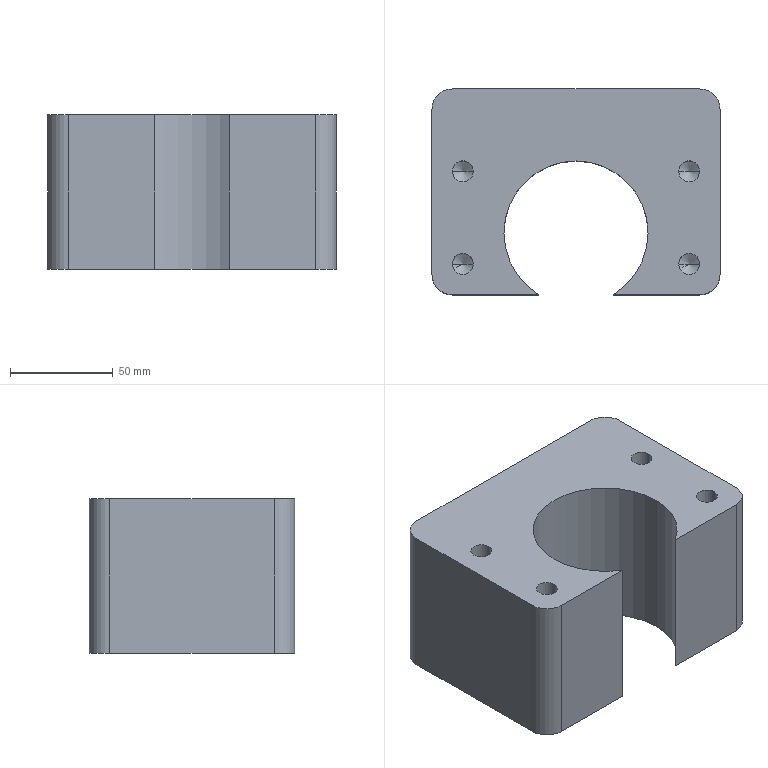Part | SolidWorks | features BaseBody 1 | 1 solid | 46 faces | box 140 x 100 x 75 mm | volume 742034 mm3 | cylinder 23 | cone 16 | plane 7 | commonest cylinder face diameters 8.5 x8 10.2 x8 20 x4 70 x3
STEP:
#1=CARTESIAN_POINT('',(-50.,40.,10.75));
#2=VERTEX_POINT('',#1);
#3=CARTESIAN_POINT('',(-50.,40.,19.25));
#4=VERTEX_POINT('',#3);
#5=CARTESIAN_POINT('',(-50.,40.,15.));
#6=DIRECTION('',(0.,1.,0.));
#7=DIRECTION('',(0.,0.,1.));
#8=AXIS2_PLACEMENT_3D('',#5,#6,#7);
#9=CIRCLE('',#8,4.25);
#10=EDGE_CURVE('',#2,#4,#9,.T.);
#11=ORIENTED_EDGE('',*,*,#10,.F.);
#12=CARTESIAN_POINT('',(-50.,70.,10.75));
#13=VERTEX_POINT('',#12);
#14=CARTESIAN_POINT('',(-50.,70.,10.75));
#15=DIRECTION('',(0.,1.,0.));
#16=VECTOR('',#15,1000.);
#17=LINE('',#14,#16);
#18=EDGE_CURVE('',#2,#13,#17,.T.);
#19=ORIENTED_EDGE('',*,*,#18,.T.);
#20=CARTESIAN_POINT('',(-50.,70.,19.25));
#21=VERTEX_POINT('',#20);
#22=CARTESIAN_POINT('',(-50.,70.,15.));
#23=DIRECTION('',(0.,1.,0.));
#24=DIRECTION('',(0.,0.,1.));
#25=AXIS2_PLACEMENT_3D('',#22,#23,#24);
#26=CIRCLE('',#25,4.25);
#27=EDGE_CURVE('',#13,#21,#26,.T.);
#28=ORIENTED_EDGE('',*,*,#27,.T.);
#29=CARTESIAN_POINT('',(-50.,70.,19.25));
#30=DIRECTION('',(0.,1.,0.));
#31=VECTOR('',#30,1000.);
#32=LINE('',#29,#31);
#33=EDGE_CURVE('',#4,#21,#32,.T.);
#34=ORIENTED_EDGE('',*,*,#33,.F.);
#35=EDGE_LOOP('',(#11,#19,#28,#34));
#36=FACE_OUTER_BOUND('',#35,.T.);
#37=CARTESIAN_POINT('',(-50.,70.,15.));
#38=DIRECTION('',(0.,1.,0.));
#39=DIRECTION('',(0.,0.,1.));
#40=AXIS2_PLACEMENT_3D('',#37,#38,#39);
#41=CYLINDRICAL_SURFACE('',#40,4.25);
#42=ADVANCED_FACE('',(#36),#41,.F.);
#43=CARTESIAN_POINT('',(-50.,37.446,15.));
#44=VERTEX_POINT('',#43);
#45=CARTESIAN_POINT('',(-50.,40.,19.25));
#46=DIRECTION('',(0.,0.515,0.8572));
#47=VECTOR('',#46,1000.);
#48=LINE('',#45,#47);
#49=EDGE_CURVE('',#44,#4,#48,.T.);
#50=ORIENTED_EDGE('',*,*,#49,.F.);
#51=CARTESIAN_POINT('',(-50.,40.,10.75));
#52=DIRECTION('',(0.,0.515,-0.8572));
#53=VECTOR('',#52,1000.);
#54=LINE('',#51,#53);
#55=EDGE_CURVE('',#44,#2,#54,.T.);
#56=ORIENTED_EDGE('',*,*,#55,.T.);
#57=ORIENTED_EDGE('',*,*,#10,.T.);
#58=EDGE_LOOP('',(#50,#56,#57));
#59=FACE_OUTER_BOUND('',#58,.T.);
#60=CARTESIAN_POINT('',(-50.,40.,15.));
#61=DIRECTION('',(0.,1.,0.));
#62=DIRECTION('',(0.,0.,1.));
#63=AXIS2_PLACEMENT_3D('',#60,#61,#62);
#64=CONICAL_SURFACE('',#63,4.25,1.03);
#65=ADVANCED_FACE('',(#59),#64,.F.);
#66=CARTESIAN_POINT('',(-50.,40.,50.75));
#67=VERTEX_POINT('',#66);
#68=CARTESIAN_POINT('',(-50.,40.,59.25));
#69=VERTEX_POINT('',#68);
#70=CARTESIAN_POINT('',(-50.,40.,55.));
#71=DIRECTION('',(0.,1.,0.));
#72=DIRECTION('',(0.,0.,1.));
#73=AXIS2_PLACEMENT_3D('',#70,#71,#72);
#74=CIRCLE('',#73,4.25);
#75=EDGE_CURVE('',#67,#69,#74,.T.);
#76=ORIENTED_EDGE('',*,*,#75,.F.);
#77=CARTESIAN_POINT('',(-50.,70.,50.75));
#78=VERTEX_POINT('',#77);
#79=CARTESIAN_POINT('',(-50.,70.,50.75));
#80=DIRECTION('',(0.,1.,0.));
#81=VECTOR('',#80,1000.);
#82=LINE('',#79,#81);
#83=EDGE_CURVE('',#67,#78,#82,.T.);
#84=ORIENTED_EDGE('',*,*,#83,.T.);
#85=CARTESIAN_POINT('',(-50.,70.,59.25));
#86=VERTEX_POINT('',#85);
#87=CARTESIAN_POINT('',(-50.,70.,55.));
#88=DIRECTION('',(0.,1.,0.));
#89=DIRECTION('',(0.,0.,1.));
#90=AXIS2_PLACEMENT_3D('',#87,#88,#89);
#91=CIRCLE('',#90,4.25);
#92=EDGE_CURVE('',#78,#86,#91,.T.);
#93=ORIENTED_EDGE('',*,*,#92,.T.);
#94=CARTESIAN_POINT('',(-50.,70.,59.25));
#95=DIRECTION('',(0.,1.,0.));
#96=VECTOR('',#95,1000.);
#97=LINE('',#94,#96);
#98=EDGE_CURVE('',#69,#86,#97,.T.);
#99=ORIENTED_EDGE('',*,*,#98,.F.);
#100=EDGE_LOOP('',(#76,#84,#93,#99));
#101=FACE_OUTER_BOUND('',#100,.T.);
#102=CARTESIAN_POINT('',(-50.,70.,55.));
#103=DIRECTION('',(0.,1.,0.));
#104=DIRECTION('',(0.,0.,1.));
#105=AXIS2_PLACEMENT_3D('',#102,#103,#104);
#106=CYLINDRICAL_SURFACE('',#105,4.25);
#107=ADVANCED_FACE('',(#101),#106,.F.);
#108=CARTESIAN_POINT('',(-50.,37.446,55.));
#109=VERTEX_POINT('',#108);
#110=CARTESIAN_POINT('',(-50.,40.,59.25));
#111=DIRECTION('',(0.,0.515,0.8572));
#112=VECTOR('',#111,1000.);
#113=LINE('',#110,#112);
#114=EDGE_CURVE('',#109,#69,#113,.T.);
#115=ORIENTED_EDGE('',*,*,#114,.F.);
#116=CARTESIAN_POINT('',(-50.,40.,50.75));
#117=DIRECTION('',(0.,0.515,-0.8572));
#118=VECTOR('',#117,1000.);
#119=LINE('',#116,#118);
#120=EDGE_CURVE('',#109,#67,#119,.T.);
#121=ORIENTED_EDGE('',*,*,#120,.T.);
#122=ORIENTED_EDGE('',*,*,#75,.T.);
#123=EDGE_LOOP('',(#115,#121,#122));
#124=FACE_OUTER_BOUND('',#123,.T.);
#125=CARTESIAN_POINT('',(-50.,40.,55.));
#126=DIRECTION('',(0.,1.,0.));
#127=DIRECTION('',(0.,0.,1.));
#128=AXIS2_PLACEMENT_3D('',#125,#126,#127);
#129=CONICAL_SURFACE('',#128,4.25,1.03);
#130=ADVANCED_FACE('',(#124),#129,.F.);
#131=CARTESIAN_POINT('',(50.,40.,50.75));
#132=VERTEX_POINT('',#131);
#133=CARTESIAN_POINT('',(50.,40.,59.25));
#134=VERTEX_POINT('',#133);
#135=CARTESIAN_POINT('',(50.,40.,55.));
#136=DIRECTION('',(0.,1.,0.));
#137=DIRECTION('',(0.,0.,1.));
#138=AXIS2_PLACEMENT_3D('',#135,#136,#137);
#139=CIRCLE('',#138,4.25);
#140=EDGE_CURVE('',#132,#134,#139,.T.);
#141=ORIENTED_EDGE('',*,*,#140,.F.);
#142=CARTESIAN_POINT('',(50.,70.,50.75));
#143=VERTEX_POINT('',#142);
#144=CARTESIAN_POINT('',(50.,70.,50.75));
#145=DIRECTION('',(0.,1.,0.));
#146=VECTOR('',#145,1000.);
#147=LINE('',#144,#146);
#148=EDGE_CURVE('',#132,#143,#147,.T.);
#149=ORIENTED_EDGE('',*,*,#148,.T.);
#150=CARTESIAN_POINT('',(50.,70.,59.25));
#151=VERTEX_POINT('',#150);
#152=CARTESIAN_POINT('',(50.,70.,55.));
#153=DIRECTION('',(0.,1.,0.));
#154=DIRECTION('',(0.,0.,1.));
#155=AXIS2_PLACEMENT_3D('',#152,#153,#154);
#156=CIRCLE('',#155,4.25);
#157=EDGE_CURVE('',#143,#151,#156,.T.);
#158=ORIENTED_EDGE('',*,*,#157,.T.);
#159=CARTESIAN_POINT('',(50.,70.,59.25));
#160=DIRECTION('',(0.,1.,0.));
#161=VECTOR('',#160,1000.);
#162=LINE('',#159,#161);
#163=EDGE_CURVE('',#134,#151,#162,.T.);
#164=ORIENTED_EDGE('',*,*,#163,.F.);
#165=EDGE_LOOP('',(#141,#149,#158,#164));
#166=FACE_OUTER_BOUND('',#165,.T.);
#167=CARTESIAN_POINT('',(50.,70.,55.));
#168=DIRECTION('',(0.,1.,0.));
#169=DIRECTION('',(0.,0.,1.));
#170=AXIS2_PLACEMENT_3D('',#167,#168,#169);
#171=CYLINDRICAL_SURFACE('',#170,4.25);
#172=ADVANCED_FACE('',(#166),#171,.F.);
#173=CARTESIAN_POINT('',(50.,37.446,55.));
#174=VERTEX_POINT('',#173);
#175=CARTESIAN_POINT('',(50.,40.,59.25));
#176=DIRECTION('',(0.,0.515,0.8572));
#177=VECTOR('',#176,1000.);
#178=LINE('',#175,#177);
#179=EDGE_CURVE('',#174,#134,#178,.T.);
#180=ORIENTED_EDGE('',*,*,#179,.F.);
#181=CARTESIAN_POINT('',(50.,40.,50.75));
#182=DIRECTION('',(0.,0.515,-0.8572));
#183=VECTOR('',#182,1000.);
#184=LINE('',#181,#183);
#185=EDGE_CURVE('',#174,#132,#184,.T.);
#186=ORIENTED_EDGE('',*,*,#185,.T.);
#187=ORIENTED_EDGE('',*,*,#140,.T.);
#188=EDGE_LOOP('',(#180,#186,#187));
#189=FACE_OUTER_BOUND('',#188,.T.);
#190=CARTESIAN_POINT('',(50.,40.,55.));
#191=DIRECTION('',(0.,1.,0.));
#192=DIRECTION('',(0.,0.,1.));
#193=AXIS2_PLACEMENT_3D('',#190,#191,#192);
#194=CONICAL_SURFACE('',#193,4.25,1.03);
#195=ADVANCED_FACE('',(#189),#194,.F.);
#196=CARTESIAN_POINT('',(50.,40.,10.75));
#197=VERTEX_POINT('',#196);
#198=CARTESIAN_POINT('',(50.,40.,19.25));
#199=VERTEX_POINT('',#198);
#200=CARTESIAN_POINT('',(50.,40.,15.));
#201=DIRECTION('',(0.,1.,0.));
#202=DIRECTION('',(0.,0.,1.));
#203=AXIS2_PLACEMENT_3D('',#200,#201,#202);
#204=CIRCLE('',#203,4.25);
#205=EDGE_CURVE('',#197,#199,#204,.T.);
#206=ORIENTED_EDGE('',*,*,#205,.F.);
#207=CARTESIAN_POINT('',(50.,70.,10.75));
#208=VERTEX_POINT('',#207);
#209=CARTESIAN_POINT('',(50.,70.,10.75));
#210=DIRECTION('',(0.,1.,0.));
#211=VECTOR('',#210,1000.);
#212=LINE('',#209,#211);
#213=EDGE_CURVE('',#197,#208,#212,.T.);
#214=ORIENTED_EDGE('',*,*,#213,.T.);
#215=CARTESIAN_POINT('',(50.,70.,19.25));
#216=VERTEX_POINT('',#215);
#217=CARTESIAN_POINT('',(50.,70.,15.));
#218=DIRECTION('',(0.,1.,0.));
#219=DIRECTION('',(0.,0.,1.));
#220=AXIS2_PLACEMENT_3D('',#217,#218,#219);
#221=CIRCLE('',#220,4.25);
#222=EDGE_CURVE('',#208,#216,#221,.T.);
#223=ORIENTED_EDGE('',*,*,#222,.T.);
#224=CARTESIAN_POINT('',(50.,70.,19.25));
#225=DIRECTION('',(0.,1.,0.));
#226=VECTOR('',#225,1000.);
#227=LINE('',#224,#226);
#228=EDGE_CURVE('',#199,#216,#227,.T.);
#229=ORIENTED_EDGE('',*,*,#228,.F.);
#230=EDGE_LOOP('',(#206,#214,#223,#229));
#231=FACE_OUTER_BOUND('',#230,.T.);
#232=CARTESIAN_POINT('',(50.,70.,15.));
#233=DIRECTION('',(0.,1.,0.));
#234=DIRECTION('',(0.,0.,1.));
#235=AXIS2_PLACEMENT_3D('',#232,#233,#234);
#236=CYLINDRICAL_SURFACE('',#235,4.25);
#237=ADVANCED_FACE('',(#231),#236,.F.);
#238=CARTESIAN_POINT('',(50.,37.446,15.));
#239=VERTEX_POINT('',#238);
#240=CARTESIAN_POINT('',(50.,40.,19.25));
#241=DIRECTION('',(0.,0.515,0.8572));
#242=VECTOR('',#241,1000.);
#243=LINE('',#240,#242);
#244=EDGE_CURVE('',#239,#199,#243,.T.);
#245=ORIENTED_EDGE('',*,*,#244,.F.);
#246=CARTESIAN_POINT('',(50.,40.,10.75));
#247=DIRECTION('',(0.,0.515,-0.8572));
#248=VECTOR('',#247,1000.);
#249=LINE('',#246,#248);
#250=EDGE_CURVE('',#239,#197,#249,.T.);
#251=ORIENTED_EDGE('',*,*,#250,.T.);
#252=ORIENTED_EDGE('',*,*,#205,.T.);
#253=EDGE_LOOP('',(#245,#251,#252));
#254=FACE_OUTER_BOUND('',#253,.T.);
#255=CARTESIAN_POINT('',(50.,40.,15.));
#256=DIRECTION('',(0.,1.,0.));
#257=DIRECTION('',(0.,0.,1.));
#258=AXIS2_PLACEMENT_3D('',#255,#256,#257);
#259=CONICAL_SURFACE('',#258,4.25,1.03);
#260=ADVANCED_FACE('',(#254),#259,.F.);
#261=CARTESIAN_POINT('',(-60.1,30.,30.));
#262=VERTEX_POINT('',#261);
#263=CARTESIAN_POINT('',(-49.9,30.,30.));
#264=VERTEX_POINT('',#263);
#265=CARTESIAN_POINT('',(-55.,30.,30.));
#266=DIRECTION('',(0.,0.,1.));
#267=DIRECTION('',(1.,0.,0.));
#268=AXIS2_PLACEMENT_3D('',#265,#266,#267);
#269=CIRCLE('',#268,5.1);
#270=EDGE_CURVE('',#262,#264,#269,.T.);
#271=ORIENTED_EDGE('',*,*,#270,.F.);
#272=CARTESIAN_POINT('',(-60.1,30.,75.));
#273=VERTEX_POINT('',#272);
#274=CARTESIAN_POINT('',(-60.1,30.,75.));
#275=DIRECTION('',(0.,0.,1.));
#276=VECTOR('',#275,1000.);
#277=LINE('',#274,#276);
#278=EDGE_CURVE('',#262,#273,#277,.T.);
#279=ORIENTED_EDGE('',*,*,#278,.T.);
#280=CARTESIAN_POINT('',(-49.9,30.,75.));
#281=VERTEX_POINT('',#280);
#282=CARTESIAN_POINT('',(-55.,30.,75.));
#283=DIRECTION('',(0.,0.,1.));
#284=DIRECTION('',(1.,0.,0.));
#285=AXIS2_PLACEMENT_3D('',#282,#283,#284);
#286=CIRCLE('',#285,5.1);
#287=EDGE_CURVE('',#273,#281,#286,.T.);
#288=ORIENTED_EDGE('',*,*,#287,.T.);
#289=CARTESIAN_POINT('',(-49.9,30.,75.));
#290=DIRECTION('',(0.,0.,1.));
#291=VECTOR('',#290,1000.);
#292=LINE('',#289,#291);
#293=EDGE_CURVE('',#264,#281,#292,.T.);
#294=ORIENTED_EDGE('',*,*,#293,.F.);
#295=EDGE_LOOP('',(#271,#279,#288,#294));
#296=FACE_OUTER_BOUND('',#295,.T.);
#297=CARTESIAN_POINT('',(-55.,30.,75.));
#298=DIRECTION('',(0.,0.,1.));
#299=DIRECTION('',(1.,0.,0.));
#300=AXIS2_PLACEMENT_3D('',#297,#298,#299);
#301=CYLINDRICAL_SURFACE('',#300,5.1);
#302=ADVANCED_FACE('',(#296),#301,.F.);
#303=CARTESIAN_POINT('',(-55.,30.,26.936));
#304=VERTEX_POINT('',#303);
#305=CARTESIAN_POINT('',(-49.9,30.,30.));
#306=DIRECTION('',(0.8572,0.,0.515));
#307=VECTOR('',#306,1000.);
#308=LINE('',#305,#307);
#309=EDGE_CURVE('',#304,#264,#308,.T.);
#310=ORIENTED_EDGE('',*,*,#309,.F.);
#311=CARTESIAN_POINT('',(-60.1,30.,30.));
#312=DIRECTION('',(-0.8572,0.,0.515));
#313=VECTOR('',#312,1000.);
#314=LINE('',#311,#313);
#315=EDGE_CURVE('',#304,#262,#314,.T.);
#316=ORIENTED_EDGE('',*,*,#315,.T.);
#317=ORIENTED_EDGE('',*,*,#270,.T.);
#318=EDGE_LOOP('',(#310,#316,#317));
#319=FACE_OUTER_BOUND('',#318,.T.);
#320=CARTESIAN_POINT('',(-55.,30.,30.));
#321=DIRECTION('',(0.,0.,1.));
#322=DIRECTION('',(1.,0.,0.));
#323=AXIS2_PLACEMENT_3D('',#320,#321,#322);
#324=CONICAL_SURFACE('',#323,5.1,1.03);
#325=ADVANCED_FACE('',(#319),#324,.F.);
#326=CARTESIAN_POINT('',(-60.1,-15.,30.));
#327=VERTEX_POINT('',#326);
#328=CARTESIAN_POINT('',(-49.9,-15.,30.));
#329=VERTEX_POINT('',#328);
#330=CARTESIAN_POINT('',(-55.,-15.,30.));
#331=DIRECTION('',(0.,0.,1.));
#332=DIRECTION('',(1.,0.,0.));
#333=AXIS2_PLACEMENT_3D('',#330,#331,#332);
#334=CIRCLE('',#333,5.1);
#335=EDGE_CURVE('',#327,#329,#334,.T.);
#336=ORIENTED_EDGE('',*,*,#335,.F.);
#337=CARTESIAN_POINT('',(-60.1,-15.,75.));
#338=VERTEX_POINT('',#337);
#339=CARTESIAN_POINT('',(-60.1,-15.,75.));
#340=DIRECTION('',(0.,0.,1.));
#341=VECTOR('',#340,1000.);
#342=LINE('',#339,#341);
#343=EDGE_CURVE('',#327,#338,#342,.T.);
#344=ORIENTED_EDGE('',*,*,#343,.T.);
#345=CARTESIAN_POINT('',(-49.9,-15.,75.));
#346=VERTEX_POINT('',#345);
#347=CARTESIAN_POINT('',(-55.,-15.,75.));
#348=DIRECTION('',(0.,0.,1.));
#349=DIRECTION('',(1.,0.,0.));
#350=AXIS2_PLACEMENT_3D('',#347,#348,#349);
#351=CIRCLE('',#350,5.1);
#352=EDGE_CURVE('',#338,#346,#351,.T.);
#353=ORIENTED_EDGE('',*,*,#352,.T.);
#354=CARTESIAN_POINT('',(-49.9,-15.,75.));
#355=DIRECTION('',(0.,0.,1.));
#356=VECTOR('',#355,1000.);
#357=LINE('',#354,#356);
#358=EDGE_CURVE('',#329,#346,#357,.T.);
#359=ORIENTED_EDGE('',*,*,#358,.F.);
#360=EDGE_LOOP('',(#336,#344,#353,#359));
#361=FACE_OUTER_BOUND('',#360,.T.);
#362=CARTESIAN_POINT('',(-55.,-15.,75.));
#363=DIRECTION('',(0.,0.,1.));
#364=DIRECTION('',(1.,0.,0.));
#365=AXIS2_PLACEMENT_3D('',#362,#363,#364);
#366=CYLINDRICAL_SURFACE('',#365,5.1);
#367=ADVANCED_FACE('',(#361),#366,.F.);
#368=CARTESIAN_POINT('',(-55.,-15.,26.936));
#369=VERTEX_POINT('',#368);
#370=CARTESIAN_POINT('',(-49.9,-15.,30.));
#371=DIRECTION('',(0.8572,0.,0.515));
#372=VECTOR('',#371,1000.);
#373=LINE('',#370,#372);
#374=EDGE_CURVE('',#369,#329,#373,.T.);
#375=ORIENTED_EDGE('',*,*,#374,.F.);
#376=CARTESIAN_POINT('',(-60.1,-15.,30.));
#377=DIRECTION('',(-0.8572,0.,0.515));
#378=VECTOR('',#377,1000.);
#379=LINE('',#376,#378);
#380=EDGE_CURVE('',#369,#327,#379,.T.);
#381=ORIENTED_EDGE('',*,*,#380,.T.);
#382=ORIENTED_EDGE('',*,*,#335,.T.);
#383=EDGE_LOOP('',(#375,#381,#382));
#384=FACE_OUTER_BOUND('',#383,.T.);
#385=CARTESIAN_POINT('',(-55.,-15.,30.));
#386=DIRECTION('',(0.,0.,1.));
#387=DIRECTION('',(1.,0.,0.));
#388=AXIS2_PLACEMENT_3D('',#385,#386,#387);
#389=CONICAL_SURFACE('',#388,5.1,1.03);
#390=ADVANCED_FACE('',(#384),#389,.F.);
#391=CARTESIAN_POINT('',(49.9,-15.,30.));
#392=VERTEX_POINT('',#391);
#393=CARTESIAN_POINT('',(60.1,-15.,30.));
#394=VERTEX_POINT('',#393);
#395=CARTESIAN_POINT('',(55.,-15.,30.));
#396=DIRECTION('',(0.,0.,1.));
#397=DIRECTION('',(1.,0.,0.));
#398=AXIS2_PLACEMENT_3D('',#395,#396,#397);
#399=CIRCLE('',#398,5.1);
#400=EDGE_CURVE('',#392,#394,#399,.T.);
#401=ORIENTED_EDGE('',*,*,#400,.F.);
#402=CARTESIAN_POINT('',(49.9,-15.,75.));
#403=VERTEX_POINT('',#402);
#404=CARTESIAN_POINT('',(49.9,-15.,75.));
#405=DIRECTION('',(0.,0.,1.));
#406=VECTOR('',#405,1000.);
#407=LINE('',#404,#406);
#408=EDGE_CURVE('',#392,#403,#407,.T.);
#409=ORIENTED_EDGE('',*,*,#408,.T.);
#410=CARTESIAN_POINT('',(60.1,-15.,75.));
#411=VERTEX_POINT('',#410);
#412=CARTESIAN_POINT('',(55.,-15.,75.));
#413=DIRECTION('',(0.,0.,1.));
#414=DIRECTION('',(1.,0.,0.));
#415=AXIS2_PLACEMENT_3D('',#412,#413,#414);
#416=CIRCLE('',#415,5.1);
#417=EDGE_CURVE('',#403,#411,#416,.T.);
#418=ORIENTED_EDGE('',*,*,#417,.T.);
#419=CARTESIAN_POINT('',(60.1,-15.,75.));
#420=DIRECTION('',(0.,0.,1.));
#421=VECTOR('',#420,1000.);
#422=LINE('',#419,#421);
#423=EDGE_CURVE('',#394,#411,#422,.T.);
#424=ORIENTED_EDGE('',*,*,#423,.F.);
#425=EDGE_LOOP('',(#401,#409,#418,#424));
#426=FACE_OUTER_BOUND('',#425,.T.);
#427=CARTESIAN_POINT('',(55.,-15.,75.));
#428=DIRECTION('',(0.,0.,1.));
#429=DIRECTION('',(1.,0.,0.));
#430=AXIS2_PLACEMENT_3D('',#427,#428,#429);
#431=CYLINDRICAL_SURFACE('',#430,5.1);
#432=ADVANCED_FACE('',(#426),#431,.F.);
#433=CARTESIAN_POINT('',(55.,-15.,26.936));
#434=VERTEX_POINT('',#433);
#435=CARTESIAN_POINT('',(60.1,-15.,30.));
#436=DIRECTION('',(0.8572,0.,0.515));
#437=VECTOR('',#436,1000.);
#438=LINE('',#435,#437);
#439=EDGE_CURVE('',#434,#394,#438,.T.);
#440=ORIENTED_EDGE('',*,*,#439,.F.);
#441=CARTESIAN_POINT('',(49.9,-15.,30.));
#442=DIRECTION('',(-0.8572,0.,0.515));
#443=VECTOR('',#442,1000.);
#444=LINE('',#441,#443);
#445=EDGE_CURVE('',#434,#392,#444,.T.);
#446=ORIENTED_EDGE('',*,*,#445,.T.);
#447=ORIENTED_EDGE('',*,*,#400,.T.);
#448=EDGE_LOOP('',(#440,#446,#447));
#449=FACE_OUTER_BOUND('',#448,.T.);
#450=CARTESIAN_POINT('',(55.,-15.,30.));
#451=DIRECTION('',(0.,0.,1.));
#452=DIRECTION('',(1.,0.,0.));
#453=AXIS2_PLACEMENT_3D('',#450,#451,#452);
#454=CONICAL_SURFACE('',#453,5.1,1.03);
#455=ADVANCED_FACE('',(#449),#454,.F.);
#456=CARTESIAN_POINT('',(49.9,30.,30.));
#457=VERTEX_POINT('',#456);
#458=CARTESIAN_POINT('',(60.1,30.,30.));
#459=VERTEX_POINT('',#458);
#460=CARTESIAN_POINT('',(55.,30.,30.));
#461=DIRECTION('',(0.,0.,1.));
#462=DIRECTION('',(1.,0.,0.));
#463=AXIS2_PLACEMENT_3D('',#460,#461,#462);
#464=CIRCLE('',#463,5.1);
#465=EDGE_CURVE('',#457,#459,#464,.T.);
#466=ORIENTED_EDGE('',*,*,#465,.F.);
#467=CARTESIAN_POINT('',(49.9,30.,75.));
#468=VERTEX_POINT('',#467);
#469=CARTESIAN_POINT('',(49.9,30.,75.));
#470=DIRECTION('',(0.,0.,1.));
#471=VECTOR('',#470,1000.);
#472=LINE('',#469,#471);
#473=EDGE_CURVE('',#457,#468,#472,.T.);
#474=ORIENTED_EDGE('',*,*,#473,.T.);
#475=CARTESIAN_POINT('',(60.1,30.,75.));
#476=VERTEX_POINT('',#475);
#477=CARTESIAN_POINT('',(55.,30.,75.));
#478=DIRECTION('',(0.,0.,1.));
#479=DIRECTION('',(1.,0.,0.));
#480=AXIS2_PLACEMENT_3D('',#477,#478,#479);
#481=CIRCLE('',#480,5.1);
#482=EDGE_CURVE('',#468,#476,#481,.T.);
#483=ORIENTED_EDGE('',*,*,#482,.T.);
#484=CARTESIAN_POINT('',(60.1,30.,75.));
#485=DIRECTION('',(0.,0.,1.));
#486=VECTOR('',#485,1000.);
#487=LINE('',#484,#486);
#488=EDGE_CURVE('',#459,#476,#487,.T.);
#489=ORIENTED_EDGE('',*,*,#488,.F.);
#490=EDGE_LOOP('',(#466,#474,#483,#489));
#491=FACE_OUTER_BOUND('',#490,.T.);
#492=CARTESIAN_POINT('',(55.,30.,75.));
#493=DIRECTION('',(0.,0.,1.));
#494=DIRECTION('',(1.,0.,0.));
#495=AXIS2_PLACEMENT_3D('',#492,#493,#494);
#496=CYLINDRICAL_SURFACE('',#495,5.1);
#497=ADVANCED_FACE('',(#491),#496,.F.);
#498=CARTESIAN_POINT('',(55.,30.,26.936));
#499=VERTEX_POINT('',#498);
#500=CARTESIAN_POINT('',(60.1,30.,30.));
#501=DIRECTION('',(0.8572,0.,0.515));
#502=VECTOR('',#501,1000.);
#503=LINE('',#500,#502);
#504=EDGE_CURVE('',#499,#459,#503,.T.);
#505=ORIENTED_EDGE('',*,*,#504,.F.);
#506=CARTESIAN_POINT('',(49.9,30.,30.));
#507=DIRECTION('',(-0.8572,0.,0.515));
#508=VECTOR('',#507,1000.);
#509=LINE('',#506,#508);
#510=EDGE_CURVE('',#499,#457,#509,.T.);
#511=ORIENTED_EDGE('',*,*,#510,.T.);
#512=ORIENTED_EDGE('',*,*,#465,.T.);
#513=EDGE_LOOP('',(#505,#511,#512));
#514=FACE_OUTER_BOUND('',#513,.T.);
#515=CARTESIAN_POINT('',(55.,30.,30.));
#516=DIRECTION('',(0.,0.,1.));
#517=DIRECTION('',(1.,0.,0.));
#518=AXIS2_PLACEMENT_3D('',#515,#516,#517);
#519=CONICAL_SURFACE('',#518,5.1,1.03);
#520=ADVANCED_FACE('',(#514),#519,.F.);
#521=CARTESIAN_POINT('',(35.,0.,75.));
#522=VERTEX_POINT('',#521);
#523=CARTESIAN_POINT('',(18.028,-30.,75.));
#524=VERTEX_POINT('',#523);
#525=CARTESIAN_POINT('',(0.,0.,75.));
#526=DIRECTION('',(0.,0.,-1.));
#527=DIRECTION('',(1.,0.,0.));
#528=AXIS2_PLACEMENT_3D('',#525,#526,#527);
#529=CIRCLE('',#528,35.);
#530=EDGE_CURVE('',#522,#524,#529,.T.);
#531=ORIENTED_EDGE('',*,*,#530,.F.);
#532=CARTESIAN_POINT('',(35.,0.,0.));
#533=VERTEX_POINT('',#532);
#534=CARTESIAN_POINT('',(35.,0.,75.));
#535=DIRECTION('',(0.,0.,-1.));
#536=VECTOR('',#535,1000.);
#537=LINE('',#534,#536);
#538=EDGE_CURVE('',#522,#533,#537,.T.);
#539=ORIENTED_EDGE('',*,*,#538,.T.);
#540=CARTESIAN_POINT('',(18.028,-30.,0.));
#541=VERTEX_POINT('',#540);
#542=CARTESIAN_POINT('',(0.,0.,0.));
#543=DIRECTION('',(0.,0.,-1.));
#544=DIRECTION('',(1.,0.,0.));
#545=AXIS2_PLACEMENT_3D('',#542,#543,#544);
#546=CIRCLE('',#545,35.);
#547=EDGE_CURVE('',#533,#541,#546,.T.);
#548=ORIENTED_EDGE('',*,*,#547,.T.);
#549=CARTESIAN_POINT('',(18.028,-30.,75.));
#550=DIRECTION('',(0.,0.,-1.));
#551=VECTOR('',#550,1000.);
#552=LINE('',#549,#551);
#553=EDGE_CURVE('',#524,#541,#552,.T.);
#554=ORIENTED_EDGE('',*,*,#553,.F.);
#555=EDGE_LOOP('',(#531,#539,#548,#554));
#556=FACE_OUTER_BOUND('',#555,.T.);
#557=CARTESIAN_POINT('',(0.,0.,75.));
#558=DIRECTION('',(0.,0.,-1.));
#559=DIRECTION('',(-1.,0.,0.));
#560=AXIS2_PLACEMENT_3D('',#557,#558,#559);
#561=CYLINDRICAL_SURFACE('',#560,35.);
#562=ADVANCED_FACE('',(#556),#561,.F.);
#563=ORIENTED_EDGE('',*,*,#538,.F.);
#564=CARTESIAN_POINT('',(-35.,0.,75.));
#565=VERTEX_POINT('',#564);
#566=CARTESIAN_POINT('',(0.,0.,75.));
#567=DIRECTION('',(0.,0.,-1.));
#568=DIRECTION('',(1.,0.,0.));
#569=AXIS2_PLACEMENT_3D('',#566,#567,#568);
#570=CIRCLE('',#569,35.);
#571=EDGE_CURVE('',#565,#522,#570,.T.);
#572=ORIENTED_EDGE('',*,*,#571,.F.);
#573=CARTESIAN_POINT('',(-35.,0.,0.));
#574=VERTEX_POINT('',#573);
#575=CARTESIAN_POINT('',(-35.,0.,75.));
#576=DIRECTION('',(0.,0.,-1.));
#577=VECTOR('',#576,1000.);
#578=LINE('',#575,#577);
#579=EDGE_CURVE('',#565,#574,#578,.T.);
#580=ORIENTED_EDGE('',*,*,#579,.T.);
#581=CARTESIAN_POINT('',(0.,0.,0.));
#582=DIRECTION('',(0.,0.,-1.));
#583=DIRECTION('',(1.,0.,0.));
#584=AXIS2_PLACEMENT_3D('',#581,#582,#583);
#585=CIRCLE('',#584,35.);
#586=EDGE_CURVE('',#574,#533,#585,.T.);
#587=ORIENTED_EDGE('',*,*,#586,.T.);
#588=EDGE_LOOP('',(#563,#572,#580,#587));
#589=FACE_OUTER_BOUND('',#588,.T.);
#590=CARTESIAN_POINT('',(0.,0.,75.));
#591=DIRECTION('',(0.,0.,-1.));
#592=DIRECTION('',(-1.,0.,0.));
#593=AXIS2_PLACEMENT_3D('',#590,#591,#592);
#594=CYLINDRICAL_SURFACE('',#593,35.);
#595=ADVANCED_FACE('',(#589),#594,.F.);
#596=ORIENTED_EDGE('',*,*,#579,.F.);
#597=CARTESIAN_POINT('',(-18.028,-30.,75.));
#598=VERTEX_POINT('',#597);
#599=CARTESIAN_POINT('',(0.,0.,75.));
#600=DIRECTION('',(0.,0.,-1.));
#601=DIRECTION('',(1.,0.,0.));
#602=AXIS2_PLACEMENT_3D('',#599,#600,#601);
#603=CIRCLE('',#602,35.);
#604=EDGE_CURVE('',#598,#565,#603,.T.);
#605=ORIENTED_EDGE('',*,*,#604,.F.);
#606=CARTESIAN_POINT('',(-18.028,-30.,0.));
#607=VERTEX_POINT('',#606);
#608=CARTESIAN_POINT('',(-18.028,-30.,75.));
#609=DIRECTION('',(0.,0.,-1.));
#610=VECTOR('',#609,1000.);
#611=LINE('',#608,#610);
#612=EDGE_CURVE('',#598,#607,#611,.T.);
#613=ORIENTED_EDGE('',*,*,#612,.T.);
#614=CARTESIAN_POINT('',(0.,0.,0.));
#615=DIRECTION('',(0.,0.,-1.));
#616=DIRECTION('',(1.,0.,0.));
#617=AXIS2_PLACEMENT_3D('',#614,#615,#616);
#618=CIRCLE('',#617,35.);
#619=EDGE_CURVE('',#607,#574,#618,.T.);
#620=ORIENTED_EDGE('',*,*,#619,.T.);
#621=EDGE_LOOP('',(#596,#605,#613,#620));
#622=FACE_OUTER_BOUND('',#621,.T.);
#623=CARTESIAN_POINT('',(0.,0.,75.));
#624=DIRECTION('',(0.,0.,-1.));
#625=DIRECTION('',(-1.,0.,0.));
#626=AXIS2_PLACEMENT_3D('',#623,#624,#625);
#627=CYLINDRICAL_SURFACE('',#626,35.);
#628=ADVANCED_FACE('',(#622),#627,.F.);
#629=CARTESIAN_POINT('',(60.,-30.,0.));
#630=VERTEX_POINT('',#629);
#631=CARTESIAN_POINT('',(18.028,-30.,0.));
#632=DIRECTION('',(1.,0.,0.));
#633=VECTOR('',#632,1000.);
#634=LINE('',#631,#633);
#635=EDGE_CURVE('',#541,#630,#634,.T.);
#636=ORIENTED_EDGE('',*,*,#635,.T.);
#637=CARTESIAN_POINT('',(60.,-30.,75.));
#638=VERTEX_POINT('',#637);
#639=CARTESIAN_POINT('',(60.,-30.,75.));
#640=DIRECTION('',(0.,0.,-1.));
#641=VECTOR('',#640,1000.);
#642=LINE('',#639,#641);
#643=EDGE_CURVE('',#638,#630,#642,.T.);
#644=ORIENTED_EDGE('',*,*,#643,.F.);
#645=CARTESIAN_POINT('',(18.028,-30.,75.));
#646=DIRECTION('',(1.,0.,0.));
#647=VECTOR('',#646,1000.);
#648=LINE('',#645,#647);
#649=EDGE_CURVE('',#524,#638,#648,.T.);
#650=ORIENTED_EDGE('',*,*,#649,.F.);
#651=ORIENTED_EDGE('',*,*,#553,.T.);
#652=EDGE_LOOP('',(#636,#644,#650,#651));
#653=FACE_OUTER_BOUND('',#652,.T.);
#654=CARTESIAN_POINT('',(18.028,-30.,75.));
#655=DIRECTION('',(0.,1.,0.));
#656=DIRECTION('',(-1.,0.,0.));
#657=AXIS2_PLACEMENT_3D('',#654,#655,#656);
#658=PLANE('',#657);
#659=ADVANCED_FACE('',(#653),#658,.F.);
#660=CARTESIAN_POINT('',(70.,-20.,0.));
#661=VERTEX_POINT('',#660);
#662=CARTESIAN_POINT('',(60.,-20.,0.));
#663=DIRECTION('',(0.,0.,1.));
#664=DIRECTION('',(1.,0.,0.));
#665=AXIS2_PLACEMENT_3D('',#662,#663,#664);
#666=CIRCLE('',#665,10.);
#667=EDGE_CURVE('',#630,#661,#666,.T.);
#668=ORIENTED_EDGE('',*,*,#667,.T.);
#669=CARTESIAN_POINT('',(70.,-20.,75.));
#670=VERTEX_POINT('',#669);
#671=CARTESIAN_POINT('',(70.,-20.,75.));
#672=DIRECTION('',(0.,0.,-1.));
#673=VECTOR('',#672,1000.);
#674=LINE('',#671,#673);
#675=EDGE_CURVE('',#670,#661,#674,.T.);
#676=ORIENTED_EDGE('',*,*,#675,.F.);
#677=CARTESIAN_POINT('',(60.,-20.,75.));
#678=DIRECTION('',(0.,0.,1.));
#679=DIRECTION('',(1.,0.,0.));
#680=AXIS2_PLACEMENT_3D('',#677,#678,#679);
#681=CIRCLE('',#680,10.);
#682=EDGE_CURVE('',#638,#670,#681,.T.);
#683=ORIENTED_EDGE('',*,*,#682,.F.);
#684=ORIENTED_EDGE('',*,*,#643,.T.);
#685=EDGE_LOOP('',(#668,#676,#683,#684));
#686=FACE_OUTER_BOUND('',#685,.T.);
#687=CARTESIAN_POINT('',(60.,-20.,75.));
#688=DIRECTION('',(0.,0.,-1.));
#689=DIRECTION('',(-1.,0.,0.));
#690=AXIS2_PLACEMENT_3D('',#687,#688,#689);
#691=CYLINDRICAL_SURFACE('',#690,10.);
#692=ADVANCED_FACE('',(#686),#691,.T.);
#693=CARTESIAN_POINT('',(70.,60.,0.));
#694=VERTEX_POINT('',#693);
#695=CARTESIAN_POINT('',(70.,-20.,0.));
#696=DIRECTION('',(0.,1.,0.));
#697=VECTOR('',#696,1000.);
#698=LINE('',#695,#697);
#699=EDGE_CURVE('',#661,#694,#698,.T.);
#700=ORIENTED_EDGE('',*,*,#699,.T.);
#701=CARTESIAN_POINT('',(70.,60.,75.));
#702=VERTEX_POINT('',#701);
#703=CARTESIAN_POINT('',(70.,60.,75.));
#704=DIRECTION('',(0.,0.,-1.));
#705=VECTOR('',#704,1000.);
#706=LINE('',#703,#705);
#707=EDGE_CURVE('',#702,#694,#706,.T.);
#708=ORIENTED_EDGE('',*,*,#707,.F.);
#709=CARTESIAN_POINT('',(70.,-20.,75.));
#710=DIRECTION('',(0.,1.,0.));
#711=VECTOR('',#710,1000.);
#712=LINE('',#709,#711);
#713=EDGE_CURVE('',#670,#702,#712,.T.);
#714=ORIENTED_EDGE('',*,*,#713,.F.);
#715=ORIENTED_EDGE('',*,*,#675,.T.);
#716=EDGE_LOOP('',(#700,#708,#714,#715));
#717=FACE_OUTER_BOUND('',#716,.T.);
#718=CARTESIAN_POINT('',(70.,-20.,75.));
#719=DIRECTION('',(-1.,0.,0.));
#720=DIRECTION('',(0.,-1.,0.));
#721=AXIS2_PLACEMENT_3D('',#718,#719,#720);
#722=PLANE('',#721);
#723=ADVANCED_FACE('',(#717),#722,.F.);
#724=CARTESIAN_POINT('',(60.,70.,0.));
#725=VERTEX_POINT('',#724);
#726=CARTESIAN_POINT('',(60.,60.,0.));
#727=DIRECTION('',(0.,0.,1.));
#728=DIRECTION('',(-1.,0.,0.));
#729=AXIS2_PLACEMENT_3D('',#726,#727,#728);
#730=CIRCLE('',#729,10.);
#731=EDGE_CURVE('',#694,#725,#730,.T.);
#732=ORIENTED_EDGE('',*,*,#731,.T.);
#733=CARTESIAN_POINT('',(60.,70.,75.));
#734=VERTEX_POINT('',#733);
#735=CARTESIAN_POINT('',(60.,70.,75.));
#736=DIRECTION('',(0.,0.,-1.));
#737=VECTOR('',#736,1000.);
#738=LINE('',#735,#737);
#739=EDGE_CURVE('',#734,#725,#738,.T.);
#740=ORIENTED_EDGE('',*,*,#739,.F.);
#741=CARTESIAN_POINT('',(60.,60.,75.));
#742=DIRECTION('',(0.,0.,1.));
#743=DIRECTION('',(-1.,0.,0.));
#744=AXIS2_PLACEMENT_3D('',#741,#742,#743);
#745=CIRCLE('',#744,10.);
#746=EDGE_CURVE('',#702,#734,#745,.T.);
#747=ORIENTED_EDGE('',*,*,#746,.F.);
#748=ORIENTED_EDGE('',*,*,#707,.T.);
#749=EDGE_LOOP('',(#732,#740,#747,#748));
#750=FACE_OUTER_BOUND('',#749,.T.);
#751=CARTESIAN_POINT('',(60.,60.,75.));
#752=DIRECTION('',(0.,0.,-1.));
#753=DIRECTION('',(-1.,0.,0.));
#754=AXIS2_PLACEMENT_3D('',#751,#752,#753);
#755=CYLINDRICAL_SURFACE('',#754,10.);
#756=ADVANCED_FACE('',(#750),#755,.T.);
#757=CARTESIAN_POINT('',(-50.,70.,15.));
#758=DIRECTION('',(0.,1.,0.));
#759=DIRECTION('',(0.,0.,1.));
#760=AXIS2_PLACEMENT_3D('',#757,#758,#759);
#761=CIRCLE('',#760,4.25);
#762=EDGE_CURVE('',#21,#13,#761,.T.);
#763=ORIENTED_EDGE('',*,*,#762,.F.);
#764=ORIENTED_EDGE('',*,*,#27,.F.);
#765=EDGE_LOOP('',(#763,#764));
#766=FACE_BOUND('',#765,.T.);
#767=CARTESIAN_POINT('',(-50.,70.,55.));
#768=DIRECTION('',(0.,1.,0.));
#769=DIRECTION('',(0.,0.,1.));
#770=AXIS2_PLACEMENT_3D('',#767,#768,#769);
#771=CIRCLE('',#770,4.25);
#772=EDGE_CURVE('',#86,#78,#771,.T.);
#773=ORIENTED_EDGE('',*,*,#772,.F.);
#774=ORIENTED_EDGE('',*,*,#92,.F.);
#775=EDGE_LOOP('',(#773,#774));
#776=FACE_BOUND('',#775,.T.);
#777=CARTESIAN_POINT('',(50.,70.,55.));
#778=DIRECTION('',(0.,1.,0.));
#779=DIRECTION('',(0.,0.,1.));
#780=AXIS2_PLACEMENT_3D('',#777,#778,#779);
#781=CIRCLE('',#780,4.25);
#782=EDGE_CURVE('',#151,#143,#781,.T.);
#783=ORIENTED_EDGE('',*,*,#782,.F.);
#784=ORIENTED_EDGE('',*,*,#157,.F.);
#785=EDGE_LOOP('',(#783,#784));
#786=FACE_BOUND('',#785,.T.);
#787=CARTESIAN_POINT('',(50.,70.,15.));
#788=DIRECTION('',(0.,1.,0.));
#789=DIRECTION('',(0.,0.,1.));
#790=AXIS2_PLACEMENT_3D('',#787,#788,#789);
#791=CIRCLE('',#790,4.25);
#792=EDGE_CURVE('',#216,#208,#791,.T.);
#793=ORIENTED_EDGE('',*,*,#792,.F.);
#794=ORIENTED_EDGE('',*,*,#222,.F.);
#795=EDGE_LOOP('',(#793,#794));
#796=FACE_BOUND('',#795,.T.);
#797=CARTESIAN_POINT('',(-60.,70.,0.));
#798=VERTEX_POINT('',#797);
#799=CARTESIAN_POINT('',(-60.,70.,0.));
#800=DIRECTION('',(-1.,0.,0.));
#801=VECTOR('',#800,1000.);
#802=LINE('',#799,#801);
#803=EDGE_CURVE('',#725,#798,#802,.T.);
#804=ORIENTED_EDGE('',*,*,#803,.T.);
#805=CARTESIAN_POINT('',(-60.,70.,75.));
#806=VERTEX_POINT('',#805);
#807=CARTESIAN_POINT('',(-60.,70.,75.));
#808=DIRECTION('',(0.,0.,-1.));
#809=VECTOR('',#808,1000.);
#810=LINE('',#807,#809);
#811=EDGE_CURVE('',#806,#798,#810,.T.);
#812=ORIENTED_EDGE('',*,*,#811,.F.);
#813=CARTESIAN_POINT('',(-60.,70.,75.));
#814=DIRECTION('',(-1.,0.,0.));
#815=VECTOR('',#814,1000.);
#816=LINE('',#813,#815);
#817=EDGE_CURVE('',#734,#806,#816,.T.);
#818=ORIENTED_EDGE('',*,*,#817,.F.);
#819=ORIENTED_EDGE('',*,*,#739,.T.);
#820=EDGE_LOOP('',(#804,#812,#818,#819));
#821=FACE_OUTER_BOUND('',#820,.T.);
#822=CARTESIAN_POINT('',(-60.,70.,75.));
#823=DIRECTION('',(0.,-1.,0.));
#824=DIRECTION('',(0.,0.,-1.));
#825=AXIS2_PLACEMENT_3D('',#822,#823,#824);
#826=PLANE('',#825);
#827=ADVANCED_FACE('',(#766,#776,#786,#796,#821),#826,.F.);
#828=CARTESIAN_POINT('',(-70.,60.,0.));
#829=VERTEX_POINT('',#828);
#830=CARTESIAN_POINT('',(-60.,60.,0.));
#831=DIRECTION('',(0.,0.,1.));
#832=DIRECTION('',(-1.,0.,0.));
#833=AXIS2_PLACEMENT_3D('',#830,#831,#832);
#834=CIRCLE('',#833,10.);
#835=EDGE_CURVE('',#798,#829,#834,.T.);
#836=ORIENTED_EDGE('',*,*,#835,.T.);
#837=CARTESIAN_POINT('',(-70.,60.,75.));
#838=VERTEX_POINT('',#837);
#839=CARTESIAN_POINT('',(-70.,60.,75.));
#840=DIRECTION('',(0.,0.,-1.));
#841=VECTOR('',#840,1000.);
#842=LINE('',#839,#841);
#843=EDGE_CURVE('',#838,#829,#842,.T.);
#844=ORIENTED_EDGE('',*,*,#843,.F.);
#845=CARTESIAN_POINT('',(-60.,60.,75.));
#846=DIRECTION('',(0.,0.,1.));
#847=DIRECTION('',(-1.,0.,0.));
#848=AXIS2_PLACEMENT_3D('',#845,#846,#847);
#849=CIRCLE('',#848,10.);
#850=EDGE_CURVE('',#806,#838,#849,.T.);
#851=ORIENTED_EDGE('',*,*,#850,.F.);
#852=ORIENTED_EDGE('',*,*,#811,.T.);
#853=EDGE_LOOP('',(#836,#844,#851,#852));
#854=FACE_OUTER_BOUND('',#853,.T.);
#855=CARTESIAN_POINT('',(-60.,60.,75.));
#856=DIRECTION('',(0.,0.,-1.));
#857=DIRECTION('',(-1.,0.,0.));
#858=AXIS2_PLACEMENT_3D('',#855,#856,#857);
#859=CYLINDRICAL_SURFACE('',#858,10.);
#860=ADVANCED_FACE('',(#854),#859,.T.);
#861=CARTESIAN_POINT('',(-70.,-20.,0.));
#862=VERTEX_POINT('',#861);
#863=CARTESIAN_POINT('',(-70.,-20.,0.));
#864=DIRECTION('',(0.,-1.,0.));
#865=VECTOR('',#864,1000.);
#866=LINE('',#863,#865);
#867=EDGE_CURVE('',#829,#862,#866,.T.);
#868=ORIENTED_EDGE('',*,*,#867,.T.);
#869=CARTESIAN_POINT('',(-70.,-20.,75.));
#870=VERTEX_POINT('',#869);
#871=CARTESIAN_POINT('',(-70.,-20.,75.));
#872=DIRECTION('',(0.,0.,-1.));
#873=VECTOR('',#872,1000.);
#874=LINE('',#871,#873);
#875=EDGE_CURVE('',#870,#862,#874,.T.);
#876=ORIENTED_EDGE('',*,*,#875,.F.);
#877=CARTESIAN_POINT('',(-70.,-20.,75.));
#878=DIRECTION('',(0.,-1.,0.));
#879=VECTOR('',#878,1000.);
#880=LINE('',#877,#879);
#881=EDGE_CURVE('',#838,#870,#880,.T.);
#882=ORIENTED_EDGE('',*,*,#881,.F.);
#883=ORIENTED_EDGE('',*,*,#843,.T.);
#884=EDGE_LOOP('',(#868,#876,#882,#883));
#885=FACE_OUTER_BOUND('',#884,.T.);
#886=CARTESIAN_POINT('',(-70.,-20.,75.));
#887=DIRECTION('',(1.,0.,0.));
#888=DIRECTION('',(0.,1.,0.));
#889=AXIS2_PLACEMENT_3D('',#886,#887,#888);
#890=PLANE('',#889);
#891=ADVANCED_FACE('',(#885),#890,.F.);
#892=CARTESIAN_POINT('',(-60.,-30.,0.));
#893=VERTEX_POINT('',#892);
#894=CARTESIAN_POINT('',(-60.,-20.,0.));
#895=DIRECTION('',(0.,0.,1.));
#896=DIRECTION('',(-1.,0.,0.));
#897=AXIS2_PLACEMENT_3D('',#894,#895,#896);
#898=CIRCLE('',#897,10.);
#899=EDGE_CURVE('',#862,#893,#898,.T.);
#900=ORIENTED_EDGE('',*,*,#899,.T.);
#901=CARTESIAN_POINT('',(-60.,-30.,75.));
#902=VERTEX_POINT('',#901);
#903=CARTESIAN_POINT('',(-60.,-30.,75.));
#904=DIRECTION('',(0.,0.,-1.));
#905=VECTOR('',#904,1000.);
#906=LINE('',#903,#905);
#907=EDGE_CURVE('',#902,#893,#906,.T.);
#908=ORIENTED_EDGE('',*,*,#907,.F.);
#909=CARTESIAN_POINT('',(-60.,-20.,75.));
#910=DIRECTION('',(0.,0.,1.));
#911=DIRECTION('',(-1.,0.,0.));
#912=AXIS2_PLACEMENT_3D('',#909,#910,#911);
#913=CIRCLE('',#912,10.);
#914=EDGE_CURVE('',#870,#902,#913,.T.);
#915=ORIENTED_EDGE('',*,*,#914,.F.);
#916=ORIENTED_EDGE('',*,*,#875,.T.);
#917=EDGE_LOOP('',(#900,#908,#915,#916));
#918=FACE_OUTER_BOUND('',#917,.T.);
#919=CARTESIAN_POINT('',(-60.,-20.,75.));
#920=DIRECTION('',(0.,0.,-1.));
#921=DIRECTION('',(-1.,0.,0.));
#922=AXIS2_PLACEMENT_3D('',#919,#920,#921);
#923=CYLINDRICAL_SURFACE('',#922,10.);
#924=ADVANCED_FACE('',(#918),#923,.T.);
#925=CARTESIAN_POINT('',(-60.,-30.,0.));
#926=DIRECTION('',(1.,0.,0.));
#927=VECTOR('',#926,1000.);
#928=LINE('',#925,#927);
#929=EDGE_CURVE('',#893,#607,#928,.T.);
#930=ORIENTED_EDGE('',*,*,#929,.T.);
#931=ORIENTED_EDGE('',*,*,#612,.F.);
#932=CARTESIAN_POINT('',(-60.,-30.,75.));
#933=DIRECTION('',(1.,0.,0.));
#934=VECTOR('',#933,1000.);
#935=LINE('',#932,#934);
#936=EDGE_CURVE('',#902,#598,#935,.T.);
#937=ORIENTED_EDGE('',*,*,#936,.F.);
#938=ORIENTED_EDGE('',*,*,#907,.T.);
#939=EDGE_LOOP('',(#930,#931,#937,#938));
#940=FACE_OUTER_BOUND('',#939,.T.);
#941=CARTESIAN_POINT('',(-60.,-30.,75.));
#942=DIRECTION('',(0.,1.,0.));
#943=DIRECTION('',(-1.,0.,0.));
#944=AXIS2_PLACEMENT_3D('',#941,#942,#943);
#945=PLANE('',#944);
#946=ADVANCED_FACE('',(#940),#945,.F.);
#947=CARTESIAN_POINT('',(-55.,30.,75.));
#948=DIRECTION('',(0.,0.,1.));
#949=DIRECTION('',(1.,0.,0.));
#950=AXIS2_PLACEMENT_3D('',#947,#948,#949);
#951=CIRCLE('',#950,5.1);
#952=EDGE_CURVE('',#281,#273,#951,.T.);
#953=ORIENTED_EDGE('',*,*,#952,.F.);
#954=ORIENTED_EDGE('',*,*,#287,.F.);
#955=EDGE_LOOP('',(#953,#954));
#956=FACE_BOUND('',#955,.T.);
#957=CARTESIAN_POINT('',(-55.,-15.,75.));
#958=DIRECTION('',(0.,0.,1.));
#959=DIRECTION('',(1.,0.,0.));
#960=AXIS2_PLACEMENT_3D('',#957,#958,#959);
#961=CIRCLE('',#960,5.1);
#962=EDGE_CURVE('',#346,#338,#961,.T.);
#963=ORIENTED_EDGE('',*,*,#962,.F.);
#964=ORIENTED_EDGE('',*,*,#352,.F.);
#965=EDGE_LOOP('',(#963,#964));
#966=FACE_BOUND('',#965,.T.);
#967=CARTESIAN_POINT('',(55.,-15.,75.));
#968=DIRECTION('',(0.,0.,1.));
#969=DIRECTION('',(1.,0.,0.));
#970=AXIS2_PLACEMENT_3D('',#967,#968,#969);
#971=CIRCLE('',#970,5.1);
#972=EDGE_CURVE('',#411,#403,#971,.T.);
#973=ORIENTED_EDGE('',*,*,#972,.F.);
#974=ORIENTED_EDGE('',*,*,#417,.F.);
#975=EDGE_LOOP('',(#973,#974));
#976=FACE_BOUND('',#975,.T.);
#977=CARTESIAN_POINT('',(55.,30.,75.));
#978=DIRECTION('',(0.,0.,1.));
#979=DIRECTION('',(1.,0.,0.));
#980=AXIS2_PLACEMENT_3D('',#977,#978,#979);
#981=CIRCLE('',#980,5.1);
#982=EDGE_CURVE('',#476,#468,#981,.T.);
#983=ORIENTED_EDGE('',*,*,#982,.F.);
#984=ORIENTED_EDGE('',*,*,#482,.F.);
#985=EDGE_LOOP('',(#983,#984));
#986=FACE_BOUND('',#985,.T.);
#987=ORIENTED_EDGE('',*,*,#604,.T.);
#988=ORIENTED_EDGE('',*,*,#571,.T.);
#989=ORIENTED_EDGE('',*,*,#530,.T.);
#990=ORIENTED_EDGE('',*,*,#649,.T.);
#991=ORIENTED_EDGE('',*,*,#682,.T.);
#992=ORIENTED_EDGE('',*,*,#713,.T.);
#993=ORIENTED_EDGE('',*,*,#746,.T.);
#994=ORIENTED_EDGE('',*,*,#817,.T.);
#995=ORIENTED_EDGE('',*,*,#850,.T.);
#996=ORIENTED_EDGE('',*,*,#881,.T.);
#997=ORIENTED_EDGE('',*,*,#914,.T.);
#998=ORIENTED_EDGE('',*,*,#936,.T.);
#999=EDGE_LOOP('',(#987,#988,#989,#990,#991,#992,#993,#994,#995,#996,#997,#998));
#1000=FACE_OUTER_BOUND('',#999,.T.);
#1001=CARTESIAN_POINT('',(0.,0.,75.));
#1002=DIRECTION('',(0.,0.,1.));
#1003=DIRECTION('',(1.,0.,0.));
#1004=AXIS2_PLACEMENT_3D('',#1001,#1002,#1003);
#1005=PLANE('',#1004);
#1006=ADVANCED_FACE('',(#956,#966,#976,#986,#1000),#1005,.T.);
#1007=ORIENTED_EDGE('',*,*,#619,.F.);
#1008=ORIENTED_EDGE('',*,*,#929,.F.);
#1009=ORIENTED_EDGE('',*,*,#899,.F.);
#1010=ORIENTED_EDGE('',*,*,#867,.F.);
#1011=ORIENTED_EDGE('',*,*,#835,.F.);
#1012=ORIENTED_EDGE('',*,*,#803,.F.);
#1013=ORIENTED_EDGE('',*,*,#731,.F.);
#1014=ORIENTED_EDGE('',*,*,#699,.F.);
#1015=ORIENTED_EDGE('',*,*,#667,.F.);
#1016=ORIENTED_EDGE('',*,*,#635,.F.);
#1017=ORIENTED_EDGE('',*,*,#547,.F.);
#1018=ORIENTED_EDGE('',*,*,#586,.F.);
#1019=EDGE_LOOP('',(#1007,#1008,#1009,#1010,#1011,#1012,#1013,#1014,#1015,#1016,#1017,#1018));
#1020=FACE_OUTER_BOUND('',#1019,.T.);
#1021=CARTESIAN_POINT('',(0.,0.,0.));
#1022=DIRECTION('',(0.,0.,1.));
#1023=DIRECTION('',(1.,0.,0.));
#1024=AXIS2_PLACEMENT_3D('',#1021,#1022,#1023);
#1025=PLANE('',#1024);
#1026=ADVANCED_FACE('',(#1020),#1025,.F.);
#1027=ORIENTED_EDGE('',*,*,#510,.F.);
#1028=ORIENTED_EDGE('',*,*,#504,.T.);
#1029=CARTESIAN_POINT('',(55.,30.,30.));
#1030=DIRECTION('',(0.,0.,1.));
#1031=DIRECTION('',(1.,0.,0.));
#1032=AXIS2_PLACEMENT_3D('',#1029,#1030,#1031);
#1033=CIRCLE('',#1032,5.1);
#1034=EDGE_CURVE('',#459,#457,#1033,.T.);
#1035=ORIENTED_EDGE('',*,*,#1034,.T.);
#1036=EDGE_LOOP('',(#1027,#1028,#1035));
#1037=FACE_OUTER_BOUND('',#1036,.T.);
#1038=CARTESIAN_POINT('',(55.,30.,30.));
#1039=DIRECTION('',(0.,0.,1.));
#1040=DIRECTION('',(1.,0.,0.));
#1041=AXIS2_PLACEMENT_3D('',#1038,#1039,#1040);
#1042=CONICAL_SURFACE('',#1041,5.1,1.03);
#1043=ADVANCED_FACE('',(#1037),#1042,.F.);
#1044=ORIENTED_EDGE('',*,*,#473,.F.);
#1045=ORIENTED_EDGE('',*,*,#1034,.F.);
#1046=ORIENTED_EDGE('',*,*,#488,.T.);
#1047=ORIENTED_EDGE('',*,*,#982,.T.);
#1048=EDGE_LOOP('',(#1044,#1045,#1046,#1047));
#1049=FACE_OUTER_BOUND('',#1048,.T.);
#1050=CARTESIAN_POINT('',(55.,30.,75.));
#1051=DIRECTION('',(0.,0.,1.));
#1052=DIRECTION('',(1.,0.,0.));
#1053=AXIS2_PLACEMENT_3D('',#1050,#1051,#1052);
#1054=CYLINDRICAL_SURFACE('',#1053,5.1);
#1055=ADVANCED_FACE('',(#1049),#1054,.F.);
#1056=ORIENTED_EDGE('',*,*,#445,.F.);
#1057=ORIENTED_EDGE('',*,*,#439,.T.);
#1058=CARTESIAN_POINT('',(55.,-15.,30.));
#1059=DIRECTION('',(0.,0.,1.));
#1060=DIRECTION('',(1.,0.,0.));
#1061=AXIS2_PLACEMENT_3D('',#1058,#1059,#1060);
#1062=CIRCLE('',#1061,5.1);
#1063=EDGE_CURVE('',#394,#392,#1062,.T.);
#1064=ORIENTED_EDGE('',*,*,#1063,.T.);
#1065=EDGE_LOOP('',(#1056,#1057,#1064));
#1066=FACE_OUTER_BOUND('',#1065,.T.);
#1067=CARTESIAN_POINT('',(55.,-15.,30.));
#1068=DIRECTION('',(0.,0.,1.));
#1069=DIRECTION('',(1.,0.,0.));
#1070=AXIS2_PLACEMENT_3D('',#1067,#1068,#1069);
#1071=CONICAL_SURFACE('',#1070,5.1,1.03);
#1072=ADVANCED_FACE('',(#1066),#1071,.F.);
#1073=ORIENTED_EDGE('',*,*,#408,.F.);
#1074=ORIENTED_EDGE('',*,*,#1063,.F.);
#1075=ORIENTED_EDGE('',*,*,#423,.T.);
#1076=ORIENTED_EDGE('',*,*,#972,.T.);
#1077=EDGE_LOOP('',(#1073,#1074,#1075,#1076));
#1078=FACE_OUTER_BOUND('',#1077,.T.);
#1079=CARTESIAN_POINT('',(55.,-15.,75.));
#1080=DIRECTION('',(0.,0.,1.));
#1081=DIRECTION('',(1.,0.,0.));
#1082=AXIS2_PLACEMENT_3D('',#1079,#1080,#1081);
#1083=CYLINDRICAL_SURFACE('',#1082,5.1);
#1084=ADVANCED_FACE('',(#1078),#1083,.F.);
#1085=ORIENTED_EDGE('',*,*,#380,.F.);
#1086=ORIENTED_EDGE('',*,*,#374,.T.);
#1087=CARTESIAN_POINT('',(-55.,-15.,30.));
#1088=DIRECTION('',(0.,0.,1.));
#1089=DIRECTION('',(1.,0.,0.));
#1090=AXIS2_PLACEMENT_3D('',#1087,#1088,#1089);
#1091=CIRCLE('',#1090,5.1);
#1092=EDGE_CURVE('',#329,#327,#1091,.T.);
#1093=ORIENTED_EDGE('',*,*,#1092,.T.);
#1094=EDGE_LOOP('',(#1085,#1086,#1093));
#1095=FACE_OUTER_BOUND('',#1094,.T.);
#1096=CARTESIAN_POINT('',(-55.,-15.,30.));
#1097=DIRECTION('',(0.,0.,1.));
#1098=DIRECTION('',(1.,0.,0.));
#1099=AXIS2_PLACEMENT_3D('',#1096,#1097,#1098);
#1100=CONICAL_SURFACE('',#1099,5.1,1.03);
#1101=ADVANCED_FACE('',(#1095),#1100,.F.);
#1102=ORIENTED_EDGE('',*,*,#343,.F.);
#1103=ORIENTED_EDGE('',*,*,#1092,.F.);
#1104=ORIENTED_EDGE('',*,*,#358,.T.);
#1105=ORIENTED_EDGE('',*,*,#962,.T.);
#1106=EDGE_LOOP('',(#1102,#1103,#1104,#1105));
#1107=FACE_OUTER_BOUND('',#1106,.T.);
#1108=CARTESIAN_POINT('',(-55.,-15.,75.));
#1109=DIRECTION('',(0.,0.,1.));
#1110=DIRECTION('',(1.,0.,0.));
#1111=AXIS2_PLACEMENT_3D('',#1108,#1109,#1110);
#1112=CYLINDRICAL_SURFACE('',#1111,5.1);
#1113=ADVANCED_FACE('',(#1107),#1112,.F.);
#1114=ORIENTED_EDGE('',*,*,#315,.F.);
#1115=ORIENTED_EDGE('',*,*,#309,.T.);
#1116=CARTESIAN_POINT('',(-55.,30.,30.));
#1117=DIRECTION('',(0.,0.,1.));
#1118=DIRECTION('',(1.,0.,0.));
#1119=AXIS2_PLACEMENT_3D('',#1116,#1117,#1118);
#1120=CIRCLE('',#1119,5.1);
#1121=EDGE_CURVE('',#264,#262,#1120,.T.);
#1122=ORIENTED_EDGE('',*,*,#1121,.T.);
#1123=EDGE_LOOP('',(#1114,#1115,#1122));
#1124=FACE_OUTER_BOUND('',#1123,.T.);
#1125=CARTESIAN_POINT('',(-55.,30.,30.));
#1126=DIRECTION('',(0.,0.,1.));
#1127=DIRECTION('',(1.,0.,0.));
#1128=AXIS2_PLACEMENT_3D('',#1125,#1126,#1127);
#1129=CONICAL_SURFACE('',#1128,5.1,1.03);
#1130=ADVANCED_FACE('',(#1124),#1129,.F.);
#1131=ORIENTED_EDGE('',*,*,#278,.F.);
#1132=ORIENTED_EDGE('',*,*,#1121,.F.);
#1133=ORIENTED_EDGE('',*,*,#293,.T.);
#1134=ORIENTED_EDGE('',*,*,#952,.T.);
#1135=EDGE_LOOP('',(#1131,#1132,#1133,#1134));
#1136=FACE_OUTER_BOUND('',#1135,.T.);
#1137=CARTESIAN_POINT('',(-55.,30.,75.));
#1138=DIRECTION('',(0.,0.,1.));
#1139=DIRECTION('',(1.,0.,0.));
#1140=AXIS2_PLACEMENT_3D('',#1137,#1138,#1139);
#1141=CYLINDRICAL_SURFACE('',#1140,5.1);
#1142=ADVANCED_FACE('',(#1136),#1141,.F.);
#1143=ORIENTED_EDGE('',*,*,#250,.F.);
#1144=ORIENTED_EDGE('',*,*,#244,.T.);
#1145=CARTESIAN_POINT('',(50.,40.,15.));
#1146=DIRECTION('',(0.,1.,0.));
#1147=DIRECTION('',(0.,0.,1.));
#1148=AXIS2_PLACEMENT_3D('',#1145,#1146,#1147);
#1149=CIRCLE('',#1148,4.25);
#1150=EDGE_CURVE('',#199,#197,#1149,.T.);
#1151=ORIENTED_EDGE('',*,*,#1150,.T.);
#1152=EDGE_LOOP('',(#1143,#1144,#1151));
#1153=FACE_OUTER_BOUND('',#1152,.T.);
#1154=CARTESIAN_POINT('',(50.,40.,15.));
#1155=DIRECTION('',(0.,1.,0.));
#1156=DIRECTION('',(0.,0.,1.));
#1157=AXIS2_PLACEMENT_3D('',#1154,#1155,#1156);
#1158=CONICAL_SURFACE('',#1157,4.25,1.03);
#1159=ADVANCED_FACE('',(#1153),#1158,.F.);
#1160=ORIENTED_EDGE('',*,*,#213,.F.);
#1161=ORIENTED_EDGE('',*,*,#1150,.F.);
#1162=ORIENTED_EDGE('',*,*,#228,.T.);
#1163=ORIENTED_EDGE('',*,*,#792,.T.);
#1164=EDGE_LOOP('',(#1160,#1161,#1162,#1163));
#1165=FACE_OUTER_BOUND('',#1164,.T.);
#1166=CARTESIAN_POINT('',(50.,70.,15.));
#1167=DIRECTION('',(0.,1.,0.));
#1168=DIRECTION('',(0.,0.,1.));
#1169=AXIS2_PLACEMENT_3D('',#1166,#1167,#1168);
#1170=CYLINDRICAL_SURFACE('',#1169,4.25);
#1171=ADVANCED_FACE('',(#1165),#1170,.F.);
#1172=ORIENTED_EDGE('',*,*,#185,.F.);
#1173=ORIENTED_EDGE('',*,*,#179,.T.);
#1174=CARTESIAN_POINT('',(50.,40.,55.));
#1175=DIRECTION('',(0.,1.,0.));
#1176=DIRECTION('',(0.,0.,1.));
#1177=AXIS2_PLACEMENT_3D('',#1174,#1175,#1176);
#1178=CIRCLE('',#1177,4.25);
#1179=EDGE_CURVE('',#134,#132,#1178,.T.);
#1180=ORIENTED_EDGE('',*,*,#1179,.T.);
#1181=EDGE_LOOP('',(#1172,#1173,#1180));
#1182=FACE_OUTER_BOUND('',#1181,.T.);
#1183=CARTESIAN_POINT('',(50.,40.,55.));
#1184=DIRECTION('',(0.,1.,0.));
#1185=DIRECTION('',(0.,0.,1.));
#1186=AXIS2_PLACEMENT_3D('',#1183,#1184,#1185);
#1187=CONICAL_SURFACE('',#1186,4.25,1.03);
#1188=ADVANCED_FACE('',(#1182),#1187,.F.);
#1189=ORIENTED_EDGE('',*,*,#148,.F.);
#1190=ORIENTED_EDGE('',*,*,#1179,.F.);
#1191=ORIENTED_EDGE('',*,*,#163,.T.);
#1192=ORIENTED_EDGE('',*,*,#782,.T.);
#1193=EDGE_LOOP('',(#1189,#1190,#1191,#1192));
#1194=FACE_OUTER_BOUND('',#1193,.T.);
#1195=CARTESIAN_POINT('',(50.,70.,55.));
#1196=DIRECTION('',(0.,1.,0.));
#1197=DIRECTION('',(0.,0.,1.));
#1198=AXIS2_PLACEMENT_3D('',#1195,#1196,#1197);
#1199=CYLINDRICAL_SURFACE('',#1198,4.25);
#1200=ADVANCED_FACE('',(#1194),#1199,.F.);
#1201=ORIENTED_EDGE('',*,*,#120,.F.);
#1202=ORIENTED_EDGE('',*,*,#114,.T.);
#1203=CARTESIAN_POINT('',(-50.,40.,55.));
#1204=DIRECTION('',(0.,1.,0.));
#1205=DIRECTION('',(0.,0.,1.));
#1206=AXIS2_PLACEMENT_3D('',#1203,#1204,#1205);
#1207=CIRCLE('',#1206,4.25);
#1208=EDGE_CURVE('',#69,#67,#1207,.T.);
#1209=ORIENTED_EDGE('',*,*,#1208,.T.);
#1210=EDGE_LOOP('',(#1201,#1202,#1209));
#1211=FACE_OUTER_BOUND('',#1210,.T.);
#1212=CARTESIAN_POINT('',(-50.,40.,55.));
#1213=DIRECTION('',(0.,1.,0.));
#1214=DIRECTION('',(0.,0.,1.));
#1215=AXIS2_PLACEMENT_3D('',#1212,#1213,#1214);
#1216=CONICAL_SURFACE('',#1215,4.25,1.03);
#1217=ADVANCED_FACE('',(#1211),#1216,.F.);
#1218=ORIENTED_EDGE('',*,*,#83,.F.);
#1219=ORIENTED_EDGE('',*,*,#1208,.F.);
#1220=ORIENTED_EDGE('',*,*,#98,.T.);
#1221=ORIENTED_EDGE('',*,*,#772,.T.);
#1222=EDGE_LOOP('',(#1218,#1219,#1220,#1221));
#1223=FACE_OUTER_BOUND('',#1222,.T.);
#1224=CARTESIAN_POINT('',(-50.,70.,55.));
#1225=DIRECTION('',(0.,1.,0.));
#1226=DIRECTION('',(0.,0.,1.));
#1227=AXIS2_PLACEMENT_3D('',#1224,#1225,#1226);
#1228=CYLINDRICAL_SURFACE('',#1227,4.25);
#1229=ADVANCED_FACE('',(#1223),#1228,.F.);
#1230=ORIENTED_EDGE('',*,*,#55,.F.);
#1231=ORIENTED_EDGE('',*,*,#49,.T.);
#1232=CARTESIAN_POINT('',(-50.,40.,15.));
#1233=DIRECTION('',(0.,1.,0.));
#1234=DIRECTION('',(0.,0.,1.));
#1235=AXIS2_PLACEMENT_3D('',#1232,#1233,#1234);
#1236=CIRCLE('',#1235,4.25);
#1237=EDGE_CURVE('',#4,#2,#1236,.T.);
#1238=ORIENTED_EDGE('',*,*,#1237,.T.);
#1239=EDGE_LOOP('',(#1230,#1231,#1238));
#1240=FACE_OUTER_BOUND('',#1239,.T.);
#1241=CARTESIAN_POINT('',(-50.,40.,15.));
#1242=DIRECTION('',(0.,1.,0.));
#1243=DIRECTION('',(0.,0.,1.));
#1244=AXIS2_PLACEMENT_3D('',#1241,#1242,#1243);
#1245=CONICAL_SURFACE('',#1244,4.25,1.03);
#1246=ADVANCED_FACE('',(#1240),#1245,.F.);
#1247=ORIENTED_EDGE('',*,*,#18,.F.);
#1248=ORIENTED_EDGE('',*,*,#1237,.F.);
#1249=ORIENTED_EDGE('',*,*,#33,.T.);
#1250=ORIENTED_EDGE('',*,*,#762,.T.);
#1251=EDGE_LOOP('',(#1247,#1248,#1249,#1250));
#1252=FACE_OUTER_BOUND('',#1251,.T.);
#1253=CARTESIAN_POINT('',(-50.,70.,15.));
#1254=DIRECTION('',(0.,1.,0.));
#1255=DIRECTION('',(0.,0.,1.));
#1256=AXIS2_PLACEMENT_3D('',#1253,#1254,#1255);
#1257=CYLINDRICAL_SURFACE('',#1256,4.25);
#1258=ADVANCED_FACE('',(#1252),#1257,.F.);
#1259=CLOSED_SHELL('',(#42,#65,#107,#130,#172,#195,#237,#260,#302,#325,#367,#390,#432,#455,#497,#520,#562,#595,#628,#659,#692,#723,#756,#827,#860,#891,#924,#946,#1006,#1026,#1043,#1055,#1072,#1084,#1101,#1113,#1130,#1142,#1159,#1171,#1188,#1200,#1217,#1229,#1246,#1258));
#1260=MANIFOLD_SOLID_BREP('',#1259);
#1261=CARTESIAN_POINT('',(0.,0.,0.));
#1262=DIRECTION('',(0.,0.,1.));
#1263=DIRECTION('',(1.,0.,0.));
#1264=AXIS2_PLACEMENT_3D('',#1261,#1262,#1263);
#1265=(LENGTH_UNIT()NAMED_UNIT(*)SI_UNIT(.MILLI.,.METRE.));
#1266=UNCERTAINTY_MEASURE_WITH_UNIT(LENGTH_MEASURE(0.00001),#1265,'','');
#1267=(NAMED_UNIT(*)PLANE_ANGLE_UNIT()SI_UNIT($,.RADIAN.));
#1268=(NAMED_UNIT(*)SI_UNIT($,.STERADIAN.)SOLID_ANGLE_UNIT());
#1269=(GEOMETRIC_REPRESENTATION_CONTEXT(3)GLOBAL_UNCERTAINTY_ASSIGNED_CONTEXT((#1266))GLOBAL_UNIT_ASSIGNED_CONTEXT((#1265,#1267,#1268))REPRESENTATION_CONTEXT('',''));
#1270=ADVANCED_BREP_SHAPE_REPRESENTATION('',(#1260,#1264),#1269);